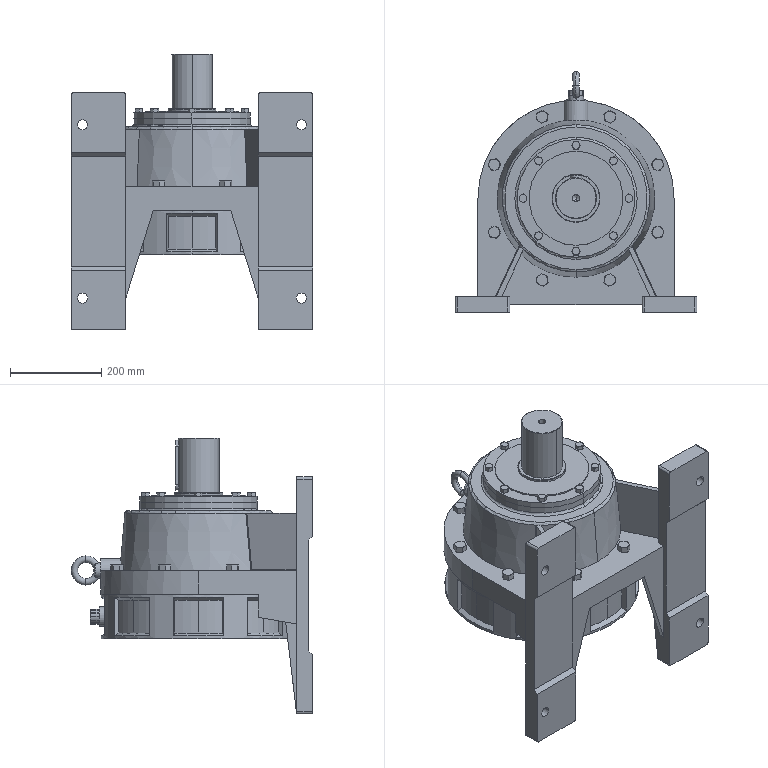Part | SolidWorks | features BaseBody 2 | 2 solids | 447 faces | box 530 x 529 x 605 mm | volume 40735700 mm3 | plane 194 | cone 145 | cylinder 94 | torus 10 | spline 2 | sphere 2 | commonest cylinder face diameters 1 x19 405.269 x16 32.797 x12 10 x8 22 x8 4 x7